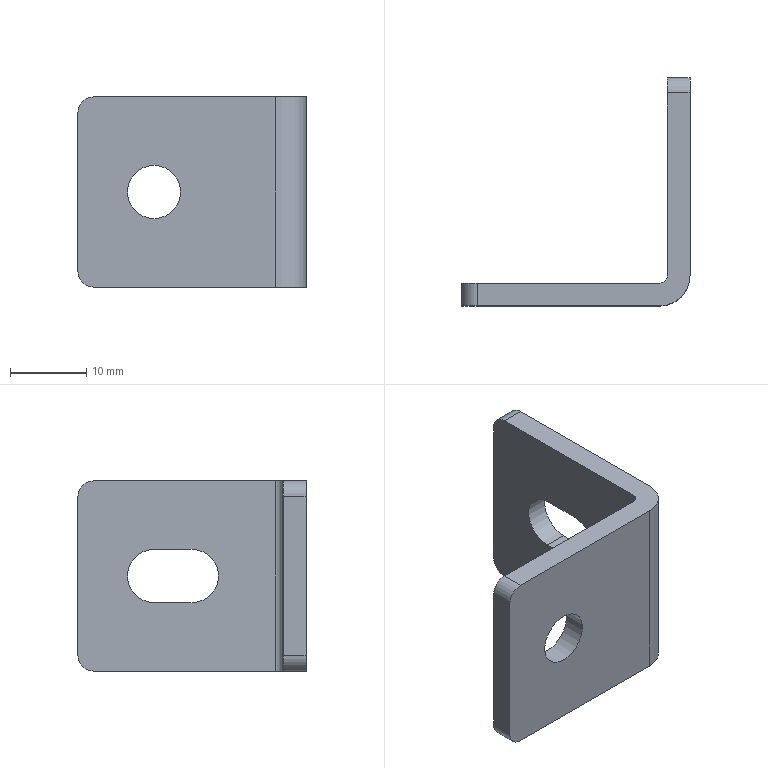Part | NX | features 5003_001_SHPTBS6 2 | 1 solid | 19 faces | box 30 x 30 x 25 mm | volume 3848 mm3 | plane 10 | cylinder 9 | commonest cylinder face diameters 4 x4 7 x3 2 x1 8 x1
STEP:
#1=CARTESIAN_POINT('',(165.825,-6.1,-131.));
#2=VERTEX_POINT('',#1);
#3=CARTESIAN_POINT('',(165.825,-6.1,-134.5));
#4=DIRECTION('',(0.,-1.,0.));
#5=DIRECTION('',(0.,0.,1.));
#6=AXIS2_PLACEMENT_3D('',#3,#4,#5);
#7=CIRCLE('',#6,3.5);
#8=EDGE_CURVE('',#2,#2,#7,.T.);
#9=ORIENTED_EDGE('',*,*,#8,.F.);
#10=EDGE_LOOP('',(#9));
#11=FACE_BOUND('',#10,.T.);
#12=CARTESIAN_POINT('',(155.825,-6.1,-124.));
#13=VERTEX_POINT('',#12);
#14=CARTESIAN_POINT('',(155.825,-6.1,-145.));
#15=VERTEX_POINT('',#14);
#16=CARTESIAN_POINT('',(155.825,-6.1,-122.));
#17=DIRECTION('',(0.,0.,-1.));
#18=VECTOR('',#17,1000.);
#19=LINE('',#16,#18);
#20=EDGE_CURVE('',#13,#15,#19,.T.);
#21=ORIENTED_EDGE('',*,*,#20,.T.);
#22=CARTESIAN_POINT('',(157.825,-6.1,-147.));
#23=VERTEX_POINT('',#22);
#24=CARTESIAN_POINT('',(157.825,-6.1,-145.));
#25=DIRECTION('',(0.,-1.,0.));
#26=DIRECTION('',(0.,0.,1.));
#27=AXIS2_PLACEMENT_3D('',#24,#25,#26);
#28=CIRCLE('',#27,2.);
#29=EDGE_CURVE('',#15,#23,#28,.T.);
#30=ORIENTED_EDGE('',*,*,#29,.T.);
#31=CARTESIAN_POINT('',(181.825,-6.1,-147.));
#32=VERTEX_POINT('',#31);
#33=CARTESIAN_POINT('',(181.825,-6.1,-147.));
#34=DIRECTION('',(-1.,0.,0.));
#35=VECTOR('',#34,1000.);
#36=LINE('',#33,#35);
#37=EDGE_CURVE('',#32,#23,#36,.T.);
#38=ORIENTED_EDGE('',*,*,#37,.F.);
#39=CARTESIAN_POINT('',(181.825,-6.1,-122.));
#40=VERTEX_POINT('',#39);
#41=CARTESIAN_POINT('',(181.825,-6.1,-122.));
#42=DIRECTION('',(0.,0.,-1.));
#43=VECTOR('',#42,1000.);
#44=LINE('',#41,#43);
#45=EDGE_CURVE('',#40,#32,#44,.T.);
#46=ORIENTED_EDGE('',*,*,#45,.F.);
#47=CARTESIAN_POINT('',(157.825,-6.1,-122.));
#48=VERTEX_POINT('',#47);
#49=CARTESIAN_POINT('',(181.825,-6.1,-122.));
#50=DIRECTION('',(-1.,0.,0.));
#51=VECTOR('',#50,1000.);
#52=LINE('',#49,#51);
#53=EDGE_CURVE('',#40,#48,#52,.T.);
#54=ORIENTED_EDGE('',*,*,#53,.T.);
#55=CARTESIAN_POINT('',(157.825,-6.1,-124.));
#56=DIRECTION('',(0.,-1.,0.));
#57=DIRECTION('',(0.,0.,1.));
#58=AXIS2_PLACEMENT_3D('',#55,#56,#57);
#59=CIRCLE('',#58,2.);
#60=EDGE_CURVE('',#48,#13,#59,.T.);
#61=ORIENTED_EDGE('',*,*,#60,.T.);
#62=EDGE_LOOP('',(#21,#30,#38,#46,#54,#61));
#63=FACE_BOUND('',#62,.T.);
#64=CARTESIAN_POINT('',(181.825,-6.1,-122.));
#65=DIRECTION('',(0.,-1.,0.));
#66=DIRECTION('',(0.,0.,1.));
#67=AXIS2_PLACEMENT_3D('',#64,#65,#66);
#68=PLANE('',#67);
#69=ADVANCED_FACE('',(#11,#63),#68,.T.);
#70=ORIENTED_EDGE('',*,*,#45,.T.);
#71=CARTESIAN_POINT('',(185.825,-2.1,-147.));
#72=VERTEX_POINT('',#71);
#73=CARTESIAN_POINT('',(181.825,-2.1,-147.));
#74=DIRECTION('',(0.,0.,-1.));
#75=DIRECTION('',(-1.,0.,0.));
#76=AXIS2_PLACEMENT_3D('',#73,#74,#75);
#77=CIRCLE('',#76,4.);
#78=EDGE_CURVE('',#72,#32,#77,.T.);
#79=ORIENTED_EDGE('',*,*,#78,.F.);
#80=CARTESIAN_POINT('',(185.825,-2.1,-122.));
#81=VERTEX_POINT('',#80);
#82=CARTESIAN_POINT('',(185.825,-2.1,-122.));
#83=DIRECTION('',(0.,0.,-1.));
#84=VECTOR('',#83,1000.);
#85=LINE('',#82,#84);
#86=EDGE_CURVE('',#81,#72,#85,.T.);
#87=ORIENTED_EDGE('',*,*,#86,.F.);
#88=CARTESIAN_POINT('',(181.825,-2.1,-122.));
#89=DIRECTION('',(0.,0.,-1.));
#90=DIRECTION('',(-1.,0.,0.));
#91=AXIS2_PLACEMENT_3D('',#88,#89,#90);
#92=CIRCLE('',#91,4.);
#93=EDGE_CURVE('',#81,#40,#92,.T.);
#94=ORIENTED_EDGE('',*,*,#93,.T.);
#95=EDGE_LOOP('',(#70,#79,#87,#94));
#96=FACE_BOUND('',#95,.T.);
#97=CARTESIAN_POINT('',(181.825,-2.1,-122.));
#98=DIRECTION('',(0.,0.,-1.));
#99=DIRECTION('',(-1.,0.,0.));
#100=AXIS2_PLACEMENT_3D('',#97,#98,#99);
#101=CYLINDRICAL_SURFACE('',#100,4.);
#102=ADVANCED_FACE('',(#96),#101,.T.);
#103=CARTESIAN_POINT('',(185.825,8.9,-138.));
#104=VERTEX_POINT('',#103);
#105=CARTESIAN_POINT('',(185.825,13.9,-138.));
#106=VERTEX_POINT('',#105);
#107=CARTESIAN_POINT('',(185.825,23.9,-138.));
#108=DIRECTION('',(0.,1.,0.));
#109=VECTOR('',#108,1000.);
#110=LINE('',#107,#109);
#111=EDGE_CURVE('',#104,#106,#110,.T.);
#112=ORIENTED_EDGE('',*,*,#111,.F.);
#113=CARTESIAN_POINT('',(185.825,8.9,-131.));
#114=VERTEX_POINT('',#113);
#115=CARTESIAN_POINT('',(185.825,8.9,-134.5));
#116=DIRECTION('',(1.,0.,0.));
#117=DIRECTION('',(0.,-1.,0.));
#118=AXIS2_PLACEMENT_3D('',#115,#116,#117);
#119=CIRCLE('',#118,3.5);
#120=EDGE_CURVE('',#114,#104,#119,.T.);
#121=ORIENTED_EDGE('',*,*,#120,.F.);
#122=CARTESIAN_POINT('',(185.825,13.9,-131.));
#123=VERTEX_POINT('',#122);
#124=CARTESIAN_POINT('',(185.825,23.9,-131.));
#125=DIRECTION('',(0.,-1.,0.));
#126=VECTOR('',#125,1000.);
#127=LINE('',#124,#126);
#128=EDGE_CURVE('',#123,#114,#127,.T.);
#129=ORIENTED_EDGE('',*,*,#128,.F.);
#130=CARTESIAN_POINT('',(185.825,13.9,-134.5));
#131=DIRECTION('',(1.,0.,0.));
#132=DIRECTION('',(0.,-1.,0.));
#133=AXIS2_PLACEMENT_3D('',#130,#131,#132);
#134=CIRCLE('',#133,3.5);
#135=EDGE_CURVE('',#106,#123,#134,.T.);
#136=ORIENTED_EDGE('',*,*,#135,.F.);
#137=EDGE_LOOP('',(#112,#121,#129,#136));
#138=FACE_BOUND('',#137,.T.);
#139=CARTESIAN_POINT('',(185.825,23.9,-124.));
#140=VERTEX_POINT('',#139);
#141=CARTESIAN_POINT('',(185.825,23.9,-145.));
#142=VERTEX_POINT('',#141);
#143=CARTESIAN_POINT('',(185.825,23.9,-122.));
#144=DIRECTION('',(0.,0.,-1.));
#145=VECTOR('',#144,1000.);
#146=LINE('',#143,#145);
#147=EDGE_CURVE('',#140,#142,#146,.T.);
#148=ORIENTED_EDGE('',*,*,#147,.F.);
#149=CARTESIAN_POINT('',(185.825,21.9,-122.));
#150=VERTEX_POINT('',#149);
#151=CARTESIAN_POINT('',(185.825,21.9,-124.));
#152=DIRECTION('',(1.,0.,0.));
#153=DIRECTION('',(0.,-1.,0.));
#154=AXIS2_PLACEMENT_3D('',#151,#152,#153);
#155=CIRCLE('',#154,2.);
#156=EDGE_CURVE('',#140,#150,#155,.T.);
#157=ORIENTED_EDGE('',*,*,#156,.T.);
#158=CARTESIAN_POINT('',(185.825,23.9,-122.));
#159=DIRECTION('',(0.,-1.,0.));
#160=VECTOR('',#159,1000.);
#161=LINE('',#158,#160);
#162=EDGE_CURVE('',#150,#81,#161,.T.);
#163=ORIENTED_EDGE('',*,*,#162,.T.);
#164=ORIENTED_EDGE('',*,*,#86,.T.);
#165=CARTESIAN_POINT('',(185.825,21.9,-147.));
#166=VERTEX_POINT('',#165);
#167=CARTESIAN_POINT('',(185.825,23.9,-147.));
#168=DIRECTION('',(0.,-1.,0.));
#169=VECTOR('',#168,1000.);
#170=LINE('',#167,#169);
#171=EDGE_CURVE('',#166,#72,#170,.T.);
#172=ORIENTED_EDGE('',*,*,#171,.F.);
#173=CARTESIAN_POINT('',(185.825,21.9,-145.));
#174=DIRECTION('',(1.,0.,0.));
#175=DIRECTION('',(0.,-1.,0.));
#176=AXIS2_PLACEMENT_3D('',#173,#174,#175);
#177=CIRCLE('',#176,2.);
#178=EDGE_CURVE('',#166,#142,#177,.T.);
#179=ORIENTED_EDGE('',*,*,#178,.T.);
#180=EDGE_LOOP('',(#148,#157,#163,#164,#172,#179));
#181=FACE_BOUND('',#180,.T.);
#182=CARTESIAN_POINT('',(185.825,23.9,-122.));
#183=DIRECTION('',(1.,0.,0.));
#184=DIRECTION('',(0.,-1.,0.));
#185=AXIS2_PLACEMENT_3D('',#182,#183,#184);
#186=PLANE('',#185);
#187=ADVANCED_FACE('',(#138,#181),#186,.T.);
#188=CARTESIAN_POINT('',(182.825,23.9,-124.));
#189=VERTEX_POINT('',#188);
#190=CARTESIAN_POINT('',(182.825,23.9,-145.));
#191=VERTEX_POINT('',#190);
#192=CARTESIAN_POINT('',(182.825,23.9,-122.));
#193=DIRECTION('',(0.,0.,-1.));
#194=VECTOR('',#193,1000.);
#195=LINE('',#192,#194);
#196=EDGE_CURVE('',#189,#191,#195,.T.);
#197=ORIENTED_EDGE('',*,*,#196,.F.);
#198=CARTESIAN_POINT('',(185.825,23.9,-124.));
#199=DIRECTION('',(-1.,0.,0.));
#200=VECTOR('',#199,1000.);
#201=LINE('',#198,#200);
#202=EDGE_CURVE('',#189,#140,#201,.F.);
#203=ORIENTED_EDGE('',*,*,#202,.T.);
#204=ORIENTED_EDGE('',*,*,#147,.T.);
#205=CARTESIAN_POINT('',(182.825,23.9,-145.));
#206=DIRECTION('',(-1.,0.,0.));
#207=VECTOR('',#206,1000.);
#208=LINE('',#205,#207);
#209=EDGE_CURVE('',#142,#191,#208,.T.);
#210=ORIENTED_EDGE('',*,*,#209,.T.);
#211=EDGE_LOOP('',(#197,#203,#204,#210));
#212=FACE_BOUND('',#211,.T.);
#213=CARTESIAN_POINT('',(185.825,23.9,-122.));
#214=DIRECTION('',(0.,-1.,0.));
#215=DIRECTION('',(0.,0.,1.));
#216=AXIS2_PLACEMENT_3D('',#213,#214,#215);
#217=PLANE('',#216);
#218=ADVANCED_FACE('',(#212),#217,.F.);
#219=CARTESIAN_POINT('',(182.825,8.9,-138.));
#220=VERTEX_POINT('',#219);
#221=CARTESIAN_POINT('',(182.825,13.9,-138.));
#222=VERTEX_POINT('',#221);
#223=CARTESIAN_POINT('',(182.825,8.9,-138.));
#224=DIRECTION('',(0.,1.,0.));
#225=VECTOR('',#224,1000.);
#226=LINE('',#223,#225);
#227=EDGE_CURVE('',#220,#222,#226,.T.);
#228=ORIENTED_EDGE('',*,*,#227,.T.);
#229=CARTESIAN_POINT('',(182.825,13.9,-131.));
#230=VERTEX_POINT('',#229);
#231=CARTESIAN_POINT('',(182.825,13.9,-134.5));
#232=DIRECTION('',(-1.,0.,0.));
#233=DIRECTION('',(0.,0.,1.));
#234=AXIS2_PLACEMENT_3D('',#231,#232,#233);
#235=CIRCLE('',#234,3.5);
#236=EDGE_CURVE('',#230,#222,#235,.T.);
#237=ORIENTED_EDGE('',*,*,#236,.F.);
#238=CARTESIAN_POINT('',(182.825,8.9,-131.));
#239=VERTEX_POINT('',#238);
#240=CARTESIAN_POINT('',(182.825,8.9,-131.));
#241=DIRECTION('',(0.,1.,0.));
#242=VECTOR('',#241,1000.);
#243=LINE('',#240,#242);
#244=EDGE_CURVE('',#239,#230,#243,.T.);
#245=ORIENTED_EDGE('',*,*,#244,.F.);
#246=CARTESIAN_POINT('',(182.825,8.9,-134.5));
#247=DIRECTION('',(-1.,0.,0.));
#248=DIRECTION('',(0.,0.,1.));
#249=AXIS2_PLACEMENT_3D('',#246,#247,#248);
#250=CIRCLE('',#249,3.5);
#251=EDGE_CURVE('',#220,#239,#250,.T.);
#252=ORIENTED_EDGE('',*,*,#251,.F.);
#253=EDGE_LOOP('',(#228,#237,#245,#252));
#254=FACE_BOUND('',#253,.T.);
#255=CARTESIAN_POINT('',(182.825,21.9,-122.));
#256=VERTEX_POINT('',#255);
#257=CARTESIAN_POINT('',(182.825,-2.1,-122.));
#258=VERTEX_POINT('',#257);
#259=CARTESIAN_POINT('',(182.825,23.9,-122.));
#260=DIRECTION('',(0.,-1.,0.));
#261=VECTOR('',#260,1000.);
#262=LINE('',#259,#261);
#263=EDGE_CURVE('',#256,#258,#262,.T.);
#264=ORIENTED_EDGE('',*,*,#263,.F.);
#265=CARTESIAN_POINT('',(182.825,21.9,-124.));
#266=DIRECTION('',(1.,0.,0.));
#267=DIRECTION('',(0.,-1.,0.));
#268=AXIS2_PLACEMENT_3D('',#265,#266,#267);
#269=CIRCLE('',#268,2.);
#270=EDGE_CURVE('',#256,#189,#269,.F.);
#271=ORIENTED_EDGE('',*,*,#270,.T.);
#272=ORIENTED_EDGE('',*,*,#196,.T.);
#273=CARTESIAN_POINT('',(182.825,21.9,-147.));
#274=VERTEX_POINT('',#273);
#275=CARTESIAN_POINT('',(182.825,21.9,-145.));
#276=DIRECTION('',(1.,0.,0.));
#277=DIRECTION('',(0.,-1.,0.));
#278=AXIS2_PLACEMENT_3D('',#275,#276,#277);
#279=CIRCLE('',#278,2.);
#280=EDGE_CURVE('',#191,#274,#279,.F.);
#281=ORIENTED_EDGE('',*,*,#280,.T.);
#282=CARTESIAN_POINT('',(182.825,-2.1,-147.));
#283=VERTEX_POINT('',#282);
#284=CARTESIAN_POINT('',(182.825,23.9,-147.));
#285=DIRECTION('',(0.,-1.,0.));
#286=VECTOR('',#285,1000.);
#287=LINE('',#284,#286);
#288=EDGE_CURVE('',#274,#283,#287,.T.);
#289=ORIENTED_EDGE('',*,*,#288,.T.);
#290=CARTESIAN_POINT('',(182.825,-2.1,-122.));
#291=DIRECTION('',(0.,0.,-1.));
#292=VECTOR('',#291,1000.);
#293=LINE('',#290,#292);
#294=EDGE_CURVE('',#258,#283,#293,.T.);
#295=ORIENTED_EDGE('',*,*,#294,.F.);
#296=EDGE_LOOP('',(#264,#271,#272,#281,#289,#295));
#297=FACE_BOUND('',#296,.T.);
#298=CARTESIAN_POINT('',(182.825,23.9,-122.));
#299=DIRECTION('',(1.,0.,0.));
#300=DIRECTION('',(0.,-1.,0.));
#301=AXIS2_PLACEMENT_3D('',#298,#299,#300);
#302=PLANE('',#301);
#303=ADVANCED_FACE('',(#254,#297),#302,.F.);
#304=ORIENTED_EDGE('',*,*,#294,.T.);
#305=CARTESIAN_POINT('',(181.825,-3.1,-147.));
#306=VERTEX_POINT('',#305);
#307=CARTESIAN_POINT('',(181.825,-2.1,-147.));
#308=DIRECTION('',(0.,0.,-1.));
#309=DIRECTION('',(1.,0.,0.));
#310=AXIS2_PLACEMENT_3D('',#307,#308,#309);
#311=CIRCLE('',#310,1.);
#312=EDGE_CURVE('',#283,#306,#311,.T.);
#313=ORIENTED_EDGE('',*,*,#312,.T.);
#314=CARTESIAN_POINT('',(181.825,-3.1,-122.));
#315=VERTEX_POINT('',#314);
#316=CARTESIAN_POINT('',(181.825,-3.1,-122.));
#317=DIRECTION('',(0.,0.,-1.));
#318=VECTOR('',#317,1000.);
#319=LINE('',#316,#318);
#320=EDGE_CURVE('',#315,#306,#319,.T.);
#321=ORIENTED_EDGE('',*,*,#320,.F.);
#322=CARTESIAN_POINT('',(181.825,-2.1,-122.));
#323=DIRECTION('',(0.,0.,-1.));
#324=DIRECTION('',(1.,0.,0.));
#325=AXIS2_PLACEMENT_3D('',#322,#323,#324);
#326=CIRCLE('',#325,1.);
#327=EDGE_CURVE('',#258,#315,#326,.T.);
#328=ORIENTED_EDGE('',*,*,#327,.F.);
#329=EDGE_LOOP('',(#304,#313,#321,#328));
#330=FACE_BOUND('',#329,.T.);
#331=CARTESIAN_POINT('',(181.825,-2.1,-122.));
#332=DIRECTION('',(0.,0.,-1.));
#333=DIRECTION('',(-1.,0.,0.));
#334=AXIS2_PLACEMENT_3D('',#331,#332,#333);
#335=CYLINDRICAL_SURFACE('',#334,1.);
#336=ADVANCED_FACE('',(#330),#335,.F.);
#337=CARTESIAN_POINT('',(165.825,-3.1,-138.));
#338=VERTEX_POINT('',#337);
#339=CARTESIAN_POINT('',(165.825,-3.1,-134.5));
#340=DIRECTION('',(0.,1.,0.));
#341=DIRECTION('',(0.,0.,-1.));
#342=AXIS2_PLACEMENT_3D('',#339,#340,#341);
#343=CIRCLE('',#342,3.5);
#344=EDGE_CURVE('',#338,#338,#343,.T.);
#345=ORIENTED_EDGE('',*,*,#344,.F.);
#346=EDGE_LOOP('',(#345));
#347=FACE_BOUND('',#346,.T.);
#348=CARTESIAN_POINT('',(157.825,-3.1,-147.));
#349=VERTEX_POINT('',#348);
#350=CARTESIAN_POINT('',(181.825,-3.1,-147.));
#351=DIRECTION('',(-1.,0.,0.));
#352=VECTOR('',#351,1000.);
#353=LINE('',#350,#352);
#354=EDGE_CURVE('',#306,#349,#353,.T.);
#355=ORIENTED_EDGE('',*,*,#354,.T.);
#356=CARTESIAN_POINT('',(155.825,-3.1,-145.));
#357=VERTEX_POINT('',#356);
#358=CARTESIAN_POINT('',(157.825,-3.1,-145.));
#359=DIRECTION('',(0.,-1.,0.));
#360=DIRECTION('',(0.,0.,1.));
#361=AXIS2_PLACEMENT_3D('',#358,#359,#360);
#362=CIRCLE('',#361,2.);
#363=EDGE_CURVE('',#349,#357,#362,.F.);
#364=ORIENTED_EDGE('',*,*,#363,.T.);
#365=CARTESIAN_POINT('',(155.825,-3.1,-124.));
#366=VERTEX_POINT('',#365);
#367=CARTESIAN_POINT('',(155.825,-3.1,-122.));
#368=DIRECTION('',(0.,0.,-1.));
#369=VECTOR('',#368,1000.);
#370=LINE('',#367,#369);
#371=EDGE_CURVE('',#366,#357,#370,.T.);
#372=ORIENTED_EDGE('',*,*,#371,.F.);
#373=CARTESIAN_POINT('',(157.825,-3.1,-122.));
#374=VERTEX_POINT('',#373);
#375=CARTESIAN_POINT('',(157.825,-3.1,-124.));
#376=DIRECTION('',(0.,-1.,0.));
#377=DIRECTION('',(0.,0.,1.));
#378=AXIS2_PLACEMENT_3D('',#375,#376,#377);
#379=CIRCLE('',#378,2.);
#380=EDGE_CURVE('',#366,#374,#379,.F.);
#381=ORIENTED_EDGE('',*,*,#380,.T.);
#382=CARTESIAN_POINT('',(181.825,-3.1,-122.));
#383=DIRECTION('',(-1.,0.,0.));
#384=VECTOR('',#383,1000.);
#385=LINE('',#382,#384);
#386=EDGE_CURVE('',#315,#374,#385,.T.);
#387=ORIENTED_EDGE('',*,*,#386,.F.);
#388=ORIENTED_EDGE('',*,*,#320,.T.);
#389=EDGE_LOOP('',(#355,#364,#372,#381,#387,#388));
#390=FACE_BOUND('',#389,.T.);
#391=CARTESIAN_POINT('',(181.825,-3.1,-122.));
#392=DIRECTION('',(0.,-1.,0.));
#393=DIRECTION('',(0.,0.,1.));
#394=AXIS2_PLACEMENT_3D('',#391,#392,#393);
#395=PLANE('',#394);
#396=ADVANCED_FACE('',(#347,#390),#395,.F.);
#397=ORIENTED_EDGE('',*,*,#371,.T.);
#398=CARTESIAN_POINT('',(155.825,-6.1,-145.));
#399=DIRECTION('',(0.,-1.,0.));
#400=VECTOR('',#399,1000.);
#401=LINE('',#398,#400);
#402=EDGE_CURVE('',#357,#15,#401,.T.);
#403=ORIENTED_EDGE('',*,*,#402,.T.);
#404=ORIENTED_EDGE('',*,*,#20,.F.);
#405=CARTESIAN_POINT('',(155.825,-3.1,-124.));
#406=DIRECTION('',(0.,-1.,0.));
#407=VECTOR('',#406,1000.);
#408=LINE('',#405,#407);
#409=EDGE_CURVE('',#13,#366,#408,.F.);
#410=ORIENTED_EDGE('',*,*,#409,.T.);
#411=EDGE_LOOP('',(#397,#403,#404,#410));
#412=FACE_BOUND('',#411,.T.);
#413=CARTESIAN_POINT('',(155.825,-3.1,-122.));
#414=DIRECTION('',(1.,0.,0.));
#415=DIRECTION('',(0.,0.,-1.));
#416=AXIS2_PLACEMENT_3D('',#413,#414,#415);
#417=PLANE('',#416);
#418=ADVANCED_FACE('',(#412),#417,.F.);
#419=ORIENTED_EDGE('',*,*,#386,.T.);
#420=CARTESIAN_POINT('',(157.825,-2.1,-122.));
#421=DIRECTION('',(0.,-1.,0.));
#422=VECTOR('',#421,1000.);
#423=LINE('',#420,#422);
#424=EDGE_CURVE('',#374,#48,#423,.T.);
#425=ORIENTED_EDGE('',*,*,#424,.T.);
#426=ORIENTED_EDGE('',*,*,#53,.F.);
#427=ORIENTED_EDGE('',*,*,#93,.F.);
#428=ORIENTED_EDGE('',*,*,#162,.F.);
#429=CARTESIAN_POINT('',(181.825,21.9,-122.));
#430=DIRECTION('',(-1.,0.,0.));
#431=VECTOR('',#430,1000.);
#432=LINE('',#429,#431);
#433=EDGE_CURVE('',#150,#256,#432,.T.);
#434=ORIENTED_EDGE('',*,*,#433,.T.);
#435=ORIENTED_EDGE('',*,*,#263,.T.);
#436=ORIENTED_EDGE('',*,*,#327,.T.);
#437=EDGE_LOOP('',(#419,#425,#426,#427,#428,#434,#435,#436));
#438=FACE_BOUND('',#437,.T.);
#439=CARTESIAN_POINT('',(181.825,-2.1,-122.));
#440=DIRECTION('',(0.,0.,-1.));
#441=DIRECTION('',(-1.,0.,0.));
#442=AXIS2_PLACEMENT_3D('',#439,#440,#441);
#443=PLANE('',#442);
#444=ADVANCED_FACE('',(#438),#443,.F.);
#445=ORIENTED_EDGE('',*,*,#37,.T.);
#446=CARTESIAN_POINT('',(157.825,-3.1,-147.));
#447=DIRECTION('',(0.,-1.,0.));
#448=VECTOR('',#447,1000.);
#449=LINE('',#446,#448);
#450=EDGE_CURVE('',#23,#349,#449,.F.);
#451=ORIENTED_EDGE('',*,*,#450,.T.);
#452=ORIENTED_EDGE('',*,*,#354,.F.);
#453=ORIENTED_EDGE('',*,*,#312,.F.);
#454=ORIENTED_EDGE('',*,*,#288,.F.);
#455=CARTESIAN_POINT('',(185.825,21.9,-147.));
#456=DIRECTION('',(-1.,0.,0.));
#457=VECTOR('',#456,1000.);
#458=LINE('',#455,#457);
#459=EDGE_CURVE('',#274,#166,#458,.F.);
#460=ORIENTED_EDGE('',*,*,#459,.T.);
#461=ORIENTED_EDGE('',*,*,#171,.T.);
#462=ORIENTED_EDGE('',*,*,#78,.T.);
#463=EDGE_LOOP('',(#445,#451,#452,#453,#454,#460,#461,#462));
#464=FACE_BOUND('',#463,.T.);
#465=CARTESIAN_POINT('',(181.825,-2.1,-147.));
#466=DIRECTION('',(0.,0.,-1.));
#467=DIRECTION('',(-1.,0.,0.));
#468=AXIS2_PLACEMENT_3D('',#465,#466,#467);
#469=PLANE('',#468);
#470=ADVANCED_FACE('',(#464),#469,.T.);
#471=ORIENTED_EDGE('',*,*,#135,.T.);
#472=CARTESIAN_POINT('',(182.825,13.9,-131.));
#473=DIRECTION('',(-1.,0.,0.));
#474=VECTOR('',#473,1000.);
#475=LINE('',#472,#474);
#476=EDGE_CURVE('',#230,#123,#475,.F.);
#477=ORIENTED_EDGE('',*,*,#476,.F.);
#478=ORIENTED_EDGE('',*,*,#236,.T.);
#479=CARTESIAN_POINT('',(182.825,13.9,-138.));
#480=DIRECTION('',(-1.,0.,0.));
#481=VECTOR('',#480,1000.);
#482=LINE('',#479,#481);
#483=EDGE_CURVE('',#106,#222,#482,.T.);
#484=ORIENTED_EDGE('',*,*,#483,.F.);
#485=EDGE_LOOP('',(#471,#477,#478,#484));
#486=FACE_BOUND('',#485,.T.);
#487=CARTESIAN_POINT('',(182.825,13.9,-134.5));
#488=DIRECTION('',(-1.,0.,0.));
#489=DIRECTION('',(0.,0.,1.));
#490=AXIS2_PLACEMENT_3D('',#487,#488,#489);
#491=CYLINDRICAL_SURFACE('',#490,3.5);
#492=ADVANCED_FACE('',(#486),#491,.F.);
#493=ORIENTED_EDGE('',*,*,#120,.T.);
#494=CARTESIAN_POINT('',(182.825,8.9,-138.));
#495=DIRECTION('',(-1.,0.,0.));
#496=VECTOR('',#495,1000.);
#497=LINE('',#494,#496);
#498=EDGE_CURVE('',#220,#104,#497,.F.);
#499=ORIENTED_EDGE('',*,*,#498,.F.);
#500=ORIENTED_EDGE('',*,*,#251,.T.);
#501=CARTESIAN_POINT('',(182.825,8.9,-131.));
#502=DIRECTION('',(-1.,0.,0.));
#503=VECTOR('',#502,1000.);
#504=LINE('',#501,#503);
#505=EDGE_CURVE('',#114,#239,#504,.T.);
#506=ORIENTED_EDGE('',*,*,#505,.F.);
#507=EDGE_LOOP('',(#493,#499,#500,#506));
#508=FACE_BOUND('',#507,.T.);
#509=CARTESIAN_POINT('',(182.825,8.9,-134.5));
#510=DIRECTION('',(-1.,0.,0.));
#511=DIRECTION('',(0.,0.,1.));
#512=AXIS2_PLACEMENT_3D('',#509,#510,#511);
#513=CYLINDRICAL_SURFACE('',#512,3.5);
#514=ADVANCED_FACE('',(#508),#513,.F.);
#515=ORIENTED_EDGE('',*,*,#111,.T.);
#516=ORIENTED_EDGE('',*,*,#483,.T.);
#517=ORIENTED_EDGE('',*,*,#227,.F.);
#518=ORIENTED_EDGE('',*,*,#498,.T.);
#519=EDGE_LOOP('',(#515,#516,#517,#518));
#520=FACE_BOUND('',#519,.T.);
#521=CARTESIAN_POINT('',(182.825,8.9,-138.));
#522=DIRECTION('',(0.,0.,-1.));
#523=DIRECTION('',(-1.,0.,0.));
#524=AXIS2_PLACEMENT_3D('',#521,#522,#523);
#525=PLANE('',#524);
#526=ADVANCED_FACE('',(#520),#525,.F.);
#527=ORIENTED_EDGE('',*,*,#128,.T.);
#528=ORIENTED_EDGE('',*,*,#505,.T.);
#529=ORIENTED_EDGE('',*,*,#244,.T.);
#530=ORIENTED_EDGE('',*,*,#476,.T.);
#531=EDGE_LOOP('',(#527,#528,#529,#530));
#532=FACE_BOUND('',#531,.T.);
#533=CARTESIAN_POINT('',(182.825,8.9,-131.));
#534=DIRECTION('',(0.,0.,1.));
#535=DIRECTION('',(1.,0.,0.));
#536=AXIS2_PLACEMENT_3D('',#533,#534,#535);
#537=PLANE('',#536);
#538=ADVANCED_FACE('',(#532),#537,.F.);
#539=ORIENTED_EDGE('',*,*,#344,.T.);
#540=EDGE_LOOP('',(#539));
#541=FACE_BOUND('',#540,.T.);
#542=ORIENTED_EDGE('',*,*,#8,.T.);
#543=EDGE_LOOP('',(#542));
#544=FACE_BOUND('',#543,.T.);
#545=CARTESIAN_POINT('',(165.825,-3.1,-134.5));
#546=DIRECTION('',(0.,1.,0.));
#547=DIRECTION('',(0.,0.,-1.));
#548=AXIS2_PLACEMENT_3D('',#545,#546,#547);
#549=CYLINDRICAL_SURFACE('',#548,3.5);
#550=ADVANCED_FACE('',(#541,#544),#549,.F.);
#551=ORIENTED_EDGE('',*,*,#363,.F.);
#552=ORIENTED_EDGE('',*,*,#450,.F.);
#553=ORIENTED_EDGE('',*,*,#29,.F.);
#554=ORIENTED_EDGE('',*,*,#402,.F.);
#555=EDGE_LOOP('',(#551,#552,#553,#554));
#556=FACE_BOUND('',#555,.T.);
#557=CARTESIAN_POINT('',(157.825,-3.1,-145.));
#558=DIRECTION('',(0.,1.,0.));
#559=DIRECTION('',(0.,0.,-1.));
#560=AXIS2_PLACEMENT_3D('',#557,#558,#559);
#561=CYLINDRICAL_SURFACE('',#560,2.);
#562=ADVANCED_FACE('',(#556),#561,.T.);
#563=ORIENTED_EDGE('',*,*,#380,.F.);
#564=ORIENTED_EDGE('',*,*,#409,.F.);
#565=ORIENTED_EDGE('',*,*,#60,.F.);
#566=ORIENTED_EDGE('',*,*,#424,.F.);
#567=EDGE_LOOP('',(#563,#564,#565,#566));
#568=FACE_BOUND('',#567,.T.);
#569=CARTESIAN_POINT('',(157.825,-2.1,-124.));
#570=DIRECTION('',(0.,-1.,0.));
#571=DIRECTION('',(0.,0.,1.));
#572=AXIS2_PLACEMENT_3D('',#569,#570,#571);
#573=CYLINDRICAL_SURFACE('',#572,2.);
#574=ADVANCED_FACE('',(#568),#573,.T.);
#575=ORIENTED_EDGE('',*,*,#156,.F.);
#576=ORIENTED_EDGE('',*,*,#202,.F.);
#577=ORIENTED_EDGE('',*,*,#270,.F.);
#578=ORIENTED_EDGE('',*,*,#433,.F.);
#579=EDGE_LOOP('',(#575,#576,#577,#578));
#580=FACE_BOUND('',#579,.T.);
#581=CARTESIAN_POINT('',(181.825,21.9,-124.));
#582=DIRECTION('',(-1.,0.,0.));
#583=DIRECTION('',(0.,0.,1.));
#584=AXIS2_PLACEMENT_3D('',#581,#582,#583);
#585=CYLINDRICAL_SURFACE('',#584,2.);
#586=ADVANCED_FACE('',(#580),#585,.T.);
#587=ORIENTED_EDGE('',*,*,#178,.F.);
#588=ORIENTED_EDGE('',*,*,#459,.F.);
#589=ORIENTED_EDGE('',*,*,#280,.F.);
#590=ORIENTED_EDGE('',*,*,#209,.F.);
#591=EDGE_LOOP('',(#587,#588,#589,#590));
#592=FACE_BOUND('',#591,.T.);
#593=CARTESIAN_POINT('',(185.825,21.9,-145.));
#594=DIRECTION('',(1.,0.,0.));
#595=DIRECTION('',(0.,0.,-1.));
#596=AXIS2_PLACEMENT_3D('',#593,#594,#595);
#597=CYLINDRICAL_SURFACE('',#596,2.);
#598=ADVANCED_FACE('',(#592),#597,.T.);
#599=CLOSED_SHELL('',(#69,#102,#187,#218,#303,#336,#396,#418,#444,#470,#492,#514,#526,#538,#550,#562,#574,#586,#598));
#600=MANIFOLD_SOLID_BREP('',#599);
#601=(LENGTH_UNIT()NAMED_UNIT(*)SI_UNIT(.MILLI.,.METRE.));
#602=UNCERTAINTY_MEASURE_WITH_UNIT(LENGTH_MEASURE(0.00001),#601,'','');
#603=(NAMED_UNIT(*)PLANE_ANGLE_UNIT()SI_UNIT($,.RADIAN.));
#604=(NAMED_UNIT(*)SI_UNIT($,.STERADIAN.)SOLID_ANGLE_UNIT());
#605=(GEOMETRIC_REPRESENTATION_CONTEXT(3)GLOBAL_UNCERTAINTY_ASSIGNED_CONTEXT((#602))GLOBAL_UNIT_ASSIGNED_CONTEXT((#601,#603,#604))REPRESENTATION_CONTEXT('',''));
#606=ADVANCED_BREP_SHAPE_REPRESENTATION('',(#600),#605);